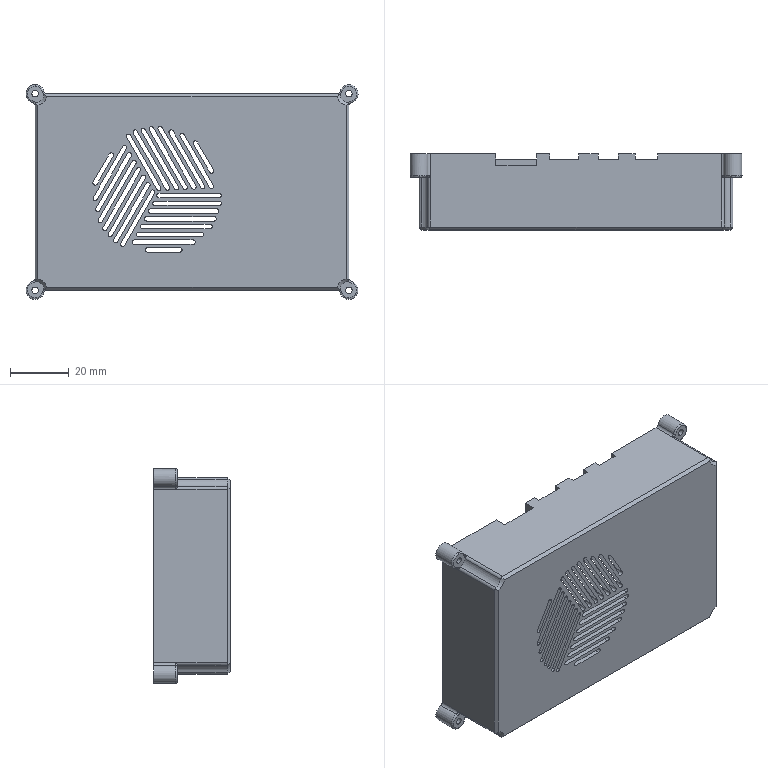Part | SolidWorks | features BaseBody 1 | 1 solid | 343 faces | box 113.2 x 26 x 73.2 mm | volume 44105 mm3 | cylinder 168 | plane 145 | spline 26 | cone 4 | commonest cylinder face diameters 2 x68 1.5 x64 6.2 x10 3.5 x9 2.2 x8 3 x4